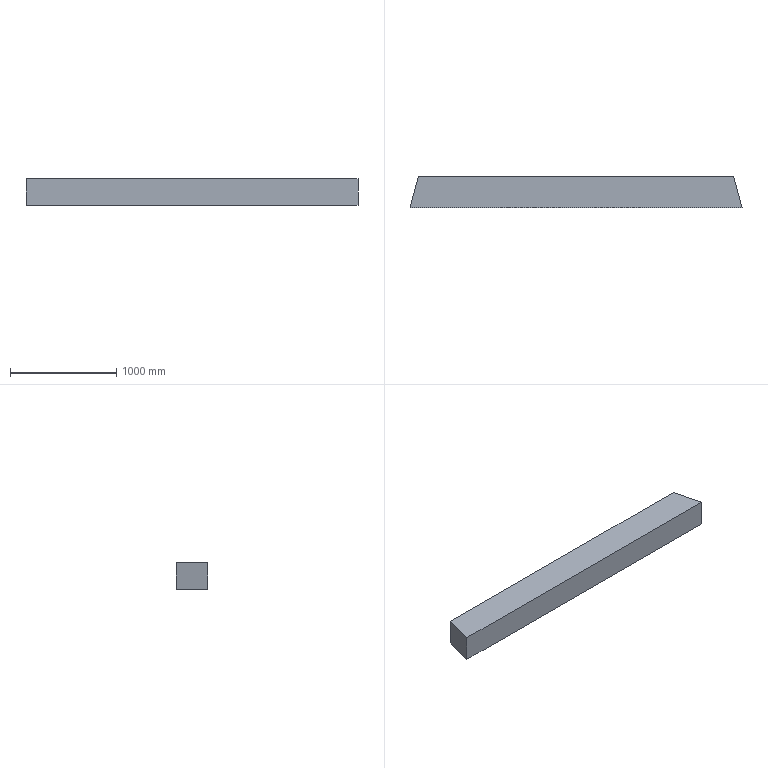Part | NX | features DATUM_CSYS 1, EXTRUDE 1, SKETCH 1 | 1 solid | 6 faces | box 3120 x 300 x 250 mm | volume 228112500 mm3 | plane 6
STEP:
#1=CARTESIAN_POINT('',(-466.,300.,-125.));
#2=VERTEX_POINT('',#1);
#3=CARTESIAN_POINT('',(-544.5,0.,-125.));
#4=VERTEX_POINT('',#3);
#5=CARTESIAN_POINT('',(-466.,300.,-125.));
#6=DIRECTION('',(-0.2531,-0.9674,0.));
#7=VECTOR('',#6,1000.);
#8=LINE('',#5,#7);
#9=EDGE_CURVE('',#2,#4,#8,.T.);
#10=ORIENTED_EDGE('',*,*,#9,.T.);
#11=CARTESIAN_POINT('',(-544.5,0.,125.));
#12=VERTEX_POINT('',#11);
#13=CARTESIAN_POINT('',(-544.5,0.,125.));
#14=DIRECTION('',(0.,0.,-1.));
#15=VECTOR('',#14,1000.);
#16=LINE('',#13,#15);
#17=EDGE_CURVE('',#12,#4,#16,.T.);
#18=ORIENTED_EDGE('',*,*,#17,.F.);
#19=CARTESIAN_POINT('',(-466.,300.,125.));
#20=VERTEX_POINT('',#19);
#21=CARTESIAN_POINT('',(-466.,300.,125.));
#22=DIRECTION('',(-0.2531,-0.9674,0.));
#23=VECTOR('',#22,1000.);
#24=LINE('',#21,#23);
#25=EDGE_CURVE('',#20,#12,#24,.T.);
#26=ORIENTED_EDGE('',*,*,#25,.F.);
#27=CARTESIAN_POINT('',(-466.,300.,125.));
#28=DIRECTION('',(0.,0.,-1.));
#29=VECTOR('',#28,1000.);
#30=LINE('',#27,#29);
#31=EDGE_CURVE('',#20,#2,#30,.T.);
#32=ORIENTED_EDGE('',*,*,#31,.T.);
#33=EDGE_LOOP('',(#10,#18,#26,#32));
#34=FACE_BOUND('',#33,.T.);
#35=CARTESIAN_POINT('',(-466.,300.,125.));
#36=DIRECTION('',(0.9674,-0.2531,0.));
#37=DIRECTION('',(0.2531,0.9674,0.));
#38=AXIS2_PLACEMENT_3D('',#35,#36,#37);
#39=PLANE('',#38);
#40=ADVANCED_FACE('',(#34),#39,.F.);
#41=CARTESIAN_POINT('',(2575.5,0.,-125.));
#42=VERTEX_POINT('',#41);
#43=CARTESIAN_POINT('',(-544.5,0.,-125.));
#44=DIRECTION('',(1.,0.,0.));
#45=VECTOR('',#44,1000.);
#46=LINE('',#43,#45);
#47=EDGE_CURVE('',#4,#42,#46,.T.);
#48=ORIENTED_EDGE('',*,*,#47,.T.);
#49=CARTESIAN_POINT('',(2575.5,0.,125.));
#50=VERTEX_POINT('',#49);
#51=CARTESIAN_POINT('',(2575.5,0.,125.));
#52=DIRECTION('',(0.,0.,-1.));
#53=VECTOR('',#52,1000.);
#54=LINE('',#51,#53);
#55=EDGE_CURVE('',#50,#42,#54,.T.);
#56=ORIENTED_EDGE('',*,*,#55,.F.);
#57=CARTESIAN_POINT('',(-544.5,0.,125.));
#58=DIRECTION('',(1.,0.,0.));
#59=VECTOR('',#58,1000.);
#60=LINE('',#57,#59);
#61=EDGE_CURVE('',#12,#50,#60,.T.);
#62=ORIENTED_EDGE('',*,*,#61,.F.);
#63=ORIENTED_EDGE('',*,*,#17,.T.);
#64=EDGE_LOOP('',(#48,#56,#62,#63));
#65=FACE_BOUND('',#64,.T.);
#66=CARTESIAN_POINT('',(-544.5,0.,125.));
#67=DIRECTION('',(0.,1.,0.));
#68=DIRECTION('',(-1.,0.,0.));
#69=AXIS2_PLACEMENT_3D('',#66,#67,#68);
#70=PLANE('',#69);
#71=ADVANCED_FACE('',(#65),#70,.F.);
#72=CARTESIAN_POINT('',(2497.,300.,-125.));
#73=VERTEX_POINT('',#72);
#74=CARTESIAN_POINT('',(2575.5,0.,-125.));
#75=DIRECTION('',(-0.2531,0.9674,0.));
#76=VECTOR('',#75,1000.);
#77=LINE('',#74,#76);
#78=EDGE_CURVE('',#42,#73,#77,.T.);
#79=ORIENTED_EDGE('',*,*,#78,.T.);
#80=CARTESIAN_POINT('',(2497.,300.,125.));
#81=VERTEX_POINT('',#80);
#82=CARTESIAN_POINT('',(2497.,300.,125.));
#83=DIRECTION('',(0.,0.,-1.));
#84=VECTOR('',#83,1000.);
#85=LINE('',#82,#84);
#86=EDGE_CURVE('',#81,#73,#85,.T.);
#87=ORIENTED_EDGE('',*,*,#86,.F.);
#88=CARTESIAN_POINT('',(2575.5,0.,125.));
#89=DIRECTION('',(-0.2531,0.9674,0.));
#90=VECTOR('',#89,1000.);
#91=LINE('',#88,#90);
#92=EDGE_CURVE('',#50,#81,#91,.T.);
#93=ORIENTED_EDGE('',*,*,#92,.F.);
#94=ORIENTED_EDGE('',*,*,#55,.T.);
#95=EDGE_LOOP('',(#79,#87,#93,#94));
#96=FACE_BOUND('',#95,.T.);
#97=CARTESIAN_POINT('',(2575.5,0.,125.));
#98=DIRECTION('',(-0.9674,-0.2531,0.));
#99=DIRECTION('',(0.2531,-0.9674,0.));
#100=AXIS2_PLACEMENT_3D('',#97,#98,#99);
#101=PLANE('',#100);
#102=ADVANCED_FACE('',(#96),#101,.F.);
#103=CARTESIAN_POINT('',(2497.,300.,-125.));
#104=DIRECTION('',(-1.,0.,0.));
#105=VECTOR('',#104,1000.);
#106=LINE('',#103,#105);
#107=EDGE_CURVE('',#73,#2,#106,.T.);
#108=ORIENTED_EDGE('',*,*,#107,.T.);
#109=ORIENTED_EDGE('',*,*,#31,.F.);
#110=CARTESIAN_POINT('',(2497.,300.,125.));
#111=DIRECTION('',(-1.,0.,0.));
#112=VECTOR('',#111,1000.);
#113=LINE('',#110,#112);
#114=EDGE_CURVE('',#81,#20,#113,.T.);
#115=ORIENTED_EDGE('',*,*,#114,.F.);
#116=ORIENTED_EDGE('',*,*,#86,.T.);
#117=EDGE_LOOP('',(#108,#109,#115,#116));
#118=FACE_BOUND('',#117,.T.);
#119=CARTESIAN_POINT('',(2497.,300.,125.));
#120=DIRECTION('',(0.,-1.,0.));
#121=DIRECTION('',(1.,0.,0.));
#122=AXIS2_PLACEMENT_3D('',#119,#120,#121);
#123=PLANE('',#122);
#124=ADVANCED_FACE('',(#118),#123,.F.);
#125=ORIENTED_EDGE('',*,*,#25,.T.);
#126=ORIENTED_EDGE('',*,*,#61,.T.);
#127=ORIENTED_EDGE('',*,*,#92,.T.);
#128=ORIENTED_EDGE('',*,*,#114,.T.);
#129=EDGE_LOOP('',(#125,#126,#127,#128));
#130=FACE_BOUND('',#129,.T.);
#131=CARTESIAN_POINT('',(0.,0.,125.));
#132=DIRECTION('',(0.,0.,1.));
#133=DIRECTION('',(1.,0.,0.));
#134=AXIS2_PLACEMENT_3D('',#131,#132,#133);
#135=PLANE('',#134);
#136=ADVANCED_FACE('',(#130),#135,.T.);
#137=ORIENTED_EDGE('',*,*,#9,.F.);
#138=ORIENTED_EDGE('',*,*,#107,.F.);
#139=ORIENTED_EDGE('',*,*,#78,.F.);
#140=ORIENTED_EDGE('',*,*,#47,.F.);
#141=EDGE_LOOP('',(#137,#138,#139,#140));
#142=FACE_BOUND('',#141,.T.);
#143=CARTESIAN_POINT('',(0.,0.,-125.));
#144=DIRECTION('',(0.,0.,1.));
#145=DIRECTION('',(1.,0.,0.));
#146=AXIS2_PLACEMENT_3D('',#143,#144,#145);
#147=PLANE('',#146);
#148=ADVANCED_FACE('',(#142),#147,.F.);
#149=CLOSED_SHELL('',(#40,#71,#102,#124,#136,#148));
#150=MANIFOLD_SOLID_BREP('',#149);
#151=(LENGTH_UNIT()NAMED_UNIT(*)SI_UNIT(.MILLI.,.METRE.));
#152=UNCERTAINTY_MEASURE_WITH_UNIT(LENGTH_MEASURE(0.00001),#151,'','');
#153=(NAMED_UNIT(*)PLANE_ANGLE_UNIT()SI_UNIT($,.RADIAN.));
#154=(NAMED_UNIT(*)SI_UNIT($,.STERADIAN.)SOLID_ANGLE_UNIT());
#155=(GEOMETRIC_REPRESENTATION_CONTEXT(3)GLOBAL_UNCERTAINTY_ASSIGNED_CONTEXT((#152))GLOBAL_UNIT_ASSIGNED_CONTEXT((#151,#153,#154))REPRESENTATION_CONTEXT('',''));
#156=ADVANCED_BREP_SHAPE_REPRESENTATION('',(#150),#155);